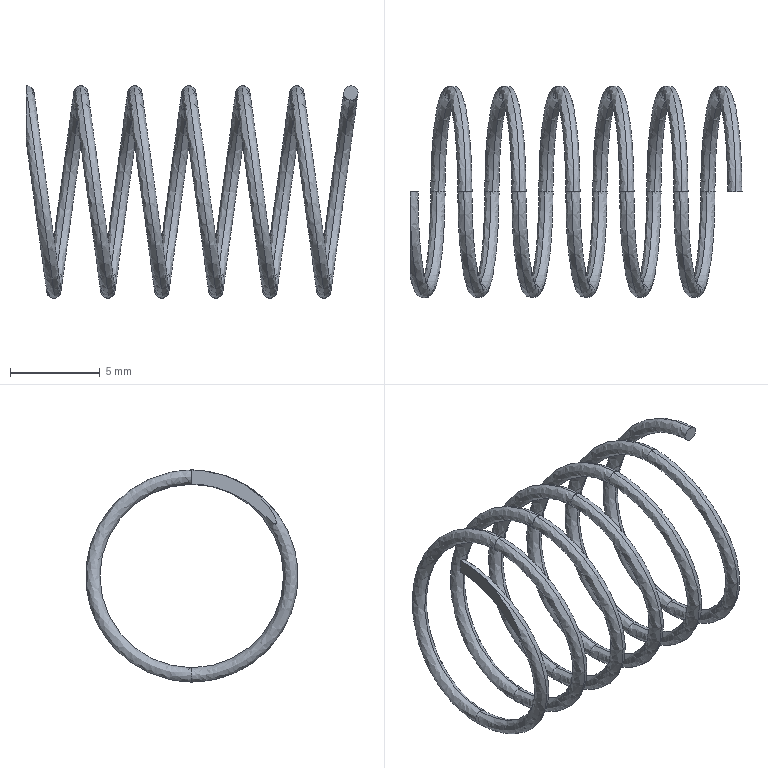Part | SolidWorks | features BaseBody 1 | 1 solid | 49 faces | box 18.454 x 11.8 x 11.8 mm | volume 104.524 mm3 | plane 25 | spline 24